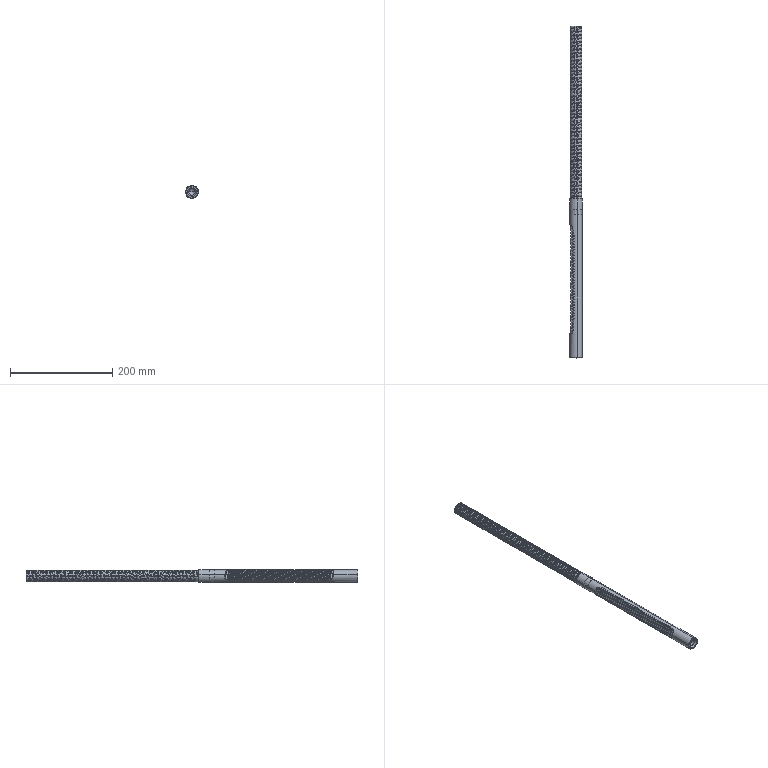Part | SolidWorks | features BaseBody 1 | 1 solid | 358 faces | box 25.15 x 648.8 x 25.15 mm | volume 264219 mm3 | plane 124 | cylinder 112 | spline 107 | cone 15 | commonest cylinder face diameters 23.2 x97 12.736 x4 24.1 x4 25.15 x4 1.762 x3